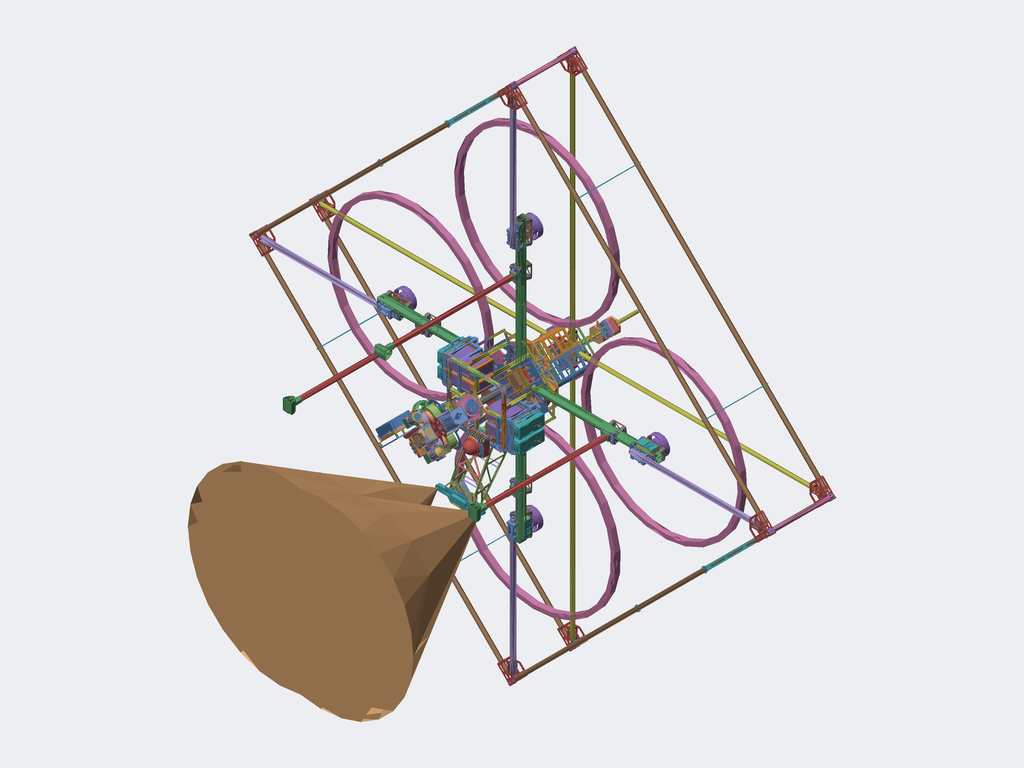Assembly | SolidWorks | 199 different items | 580 placed
Parts list (item | name | quantity | parent item | size | volume | features):
1 | 3D_PCB2_2025-12-14.step (subassembly) | x1 | - | - | - | -
2 | (subassembly) | x2 | in 9 | 27.581 x 78.075 x 26.95 mm | 6505 mm3 | -
3 | (subassembly) | x1 | in 16 | 62 x 54.7 x 76 mm | 57730 mm3 | -
4 | (subassembly) | x1 | in 14 | 113.2 x 36 x 73.2 mm | 73752 mm3 | -
5 | (subassembly) | x1 | in 16 | 72.737 x 60.097 x 64.874 mm | 142272 mm3 | -
6 | (subassembly) | x1 | in 16 | 60.743 x 60.049 x 12 mm | 6986 mm3 | -
7 | (subassembly) | x1 | in 16 | 852.82 x 786 x 692.82 mm | 107026744 mm3 | -
8 | (subassembly) | x1 | in 14 | - | - | -
9 | (subassembly) | x2 | in 16 | - | 914521 mm3 | features InContextFeatHolder 1
10 | (subassembly) | x1 | - | - | - | features InContextFeatHolder 2
11 | (subassembly) | x1 | - | - | - | features CompositeCurve 1
12 | (subassembly) | x1 | in 10 | 110.5 x 147.904 x 41 mm | 42458 mm3 | -
13 | (subassembly) | x1 | in 14 | - | 15304 mm3 | -
14 | (subassembly) | x1 | in 10 | - | - | features CenterOfMass 1
15 | (subassembly) | x1 | in 11 | - | 484779 mm3 | -
16 | (subassembly) | x1 | in 11 | - | - | features InContextFeatHolder 6, CompositeCurve 2
17 | (subassembly) | x1 | in 16 | 113.626 x 72.5 x 130.8 mm | 166546 mm3 | -
18 | BM02B-GHS-TBT.stp | x1 | - | - | - | -
19 | BM04B-GHS-TBT.stp | x1 | - | - | - | -
20 | Board~NjeS_1.step | x1 | - | - | - | -
21 | BottomSilkscreen~NjeS_1.step | x1 | - | - | - | -
22 | - | x1 | in 10 | 16 x 46 x 46 mm | 10417 mm3 | features ICE 6, CirPattern 2, Cut 1, Fillet 1, RefAxis 1, Revolution 1
23 | - | x1 | in 6 | 60 x 60 x 3 mm | 6153 mm3 | features Extrusion 1
24 | - | x32 | in 16 | 36 x 18 x 10 mm | 2888 mm3 | features Fillet 4, Extrusion 1, ICE 1
25 | - | x4 | in 16 | 36 x 3 x 88 mm | 5789 mm3 | features Fillet 3, Extrusion 1, ICE 1
26 | - | x1 | in 16 | 54 x 9.4 x 47.569 mm | 2533 mm3 | features ICE 6, Fillet 2, BossThin 1, Chamfer 1, CirPattern 1, Extrusion 1, MirrorPattern 1, Rib 1
27 | - | x1 | in 16 | 153.518 x 1.5 x 153.518 mm | 7437 mm3 | features Fillet 4, Extrusion 1, ICE 1
28 | - | x2 | in 16 | 194.5 x 58 x 2 mm | 4743 mm3 | features Fillet 5, ICE 2, Chamfer 1, Extrusion 1
29 | - | x2 | in 16 | 24 x 58 x 6.5 mm | 2190 mm3 | features ICE 2, Extrusion 1, Fillet 1
30 | - | x4 | in 16 | 24 x 31 x 24 mm | 4448 mm3 | features Extrusion 1, ICE 1
31 | - | x4 | in 16 | 137.074 x 6.5 x 56.497 mm | 3888 mm3 | features Fillet 5, ICE 3, Extrusion 1
32 | - | x4 | in 2 | 25 x 20.4 x 5.4 mm | 1256 mm3 | features ICE 2, Chamfer 1, Extrusion 1, Fillet 1
33 | - | x1 | in 10 | 22 x 68 x 68 mm | 23228 mm3 | features ICE 6, Fillet 2, BossThin 1, Chamfer 1, CirPattern 1, Cut 1, RefAxis 1, Revolution 1
34 | - | x1 | in 16 | - | 27564 mm3 | features BaseBody 46, ICE 1
35 | - | x1 | in 16 | 76 x 15.652 x 219.462 mm | 48611 mm3 | features BaseBody 13, Revolution 2, ICE 1
36 | - | x1 | in 16 | 45.5 x 41.918 x 59.598 mm | 18797 mm3 | features BaseBody 3, 3DProfileFeature 2, ICE 1, MoveCopyBody 1, NetBlend 1, RefAxis 1, Revolution 1, Sweep 1
37 | - | x1 | in 16 | 66.65 x 61 x 41.1 mm | 16016 mm3 | features ICE 15, Fillet 6, Chamfer 2, Extrusion 1, MirrorPattern 1, RevCut 1, Revolution 1
38 | - | x1 | in 16 | 20 x 140 x 20 mm | 8357 mm3 | features Extrusion 1
39 | - | x4 | in 6 | 6.928 x 6 x 12 mm | 208.267 mm3 | features ICE 2, Extrusion 1
40 | - | x1 | in 16 | 182.976 x 151.8 x 144 mm | 82758 mm3 | features Fillet 17, ICE 10, Extrusion 1, MirrorPattern 1
41 | - | x1 | in 16 | 255.002 x 2 x 157 mm | 8812 mm3 | features Extrusion 1
42 | - | x1 | in 16 | 120.4 x 151.9 x 56.149 mm | 26782 mm3 | features ICE 3, Fillet 2, Emboss 1, Extrusion 1
43 | - | x3 | in 16 | 23.98 x 1 x 7 mm | 119.201 mm3 | features Extrusion 1
44 | - | x1 | in 10 | 76.5 x 63 x 2 mm | 4222 mm3 | features Fillet 4, ICE 4, Extrusion 1
45 | - | x1 | in 16 | 238 x 19 x 238 mm | 66674 mm3 | features ICE 9, Fillet 5, MirrorPattern 3, Extrusion 1
46 | - | x4 | in 16 | 44 x 19 x 68 mm | 11985 mm3 | features ICE 11, Fillet 7, MirrorPattern 3, Extrusion 1
47 | - | x4 | in 16 | 6.889 x 27.8 x 58 mm | 3675 mm3 | features ICE 2, Extrusion 1, Fillet 1
48 | - | x4 | in 9 | 44.3 x 134.791 x 101.5 mm | 420051 mm3 | features BaseBody 9, CenterOfMass 1
49 | - | x96 | in 15, 16 | 17 x 8 x 7 mm | 450.526 mm3 | features Extrusion 1, ICE 1
50 | - | x4 | in 15 | 14 x 14 x 926.63 mm | 19619 mm3 | features Extrusion 1, ICE 1
51 | - | x4 | in 16 | 12 x 12 x 508 mm | 22307 mm3 | features ICE 2, Extrusion 1
52 | - | x4 | in 15 | 12 x 4.8 x 42 mm | 1272 mm3 | features Extrusion 1, Fillet 1
53 | - | x4 | in 16 | 36 x 2 x 88 mm | 3130 mm3 | features Fillet 3, Extrusion 1, ICE 1
54 | - | x4 | in 16 | 40.135 x 16 x 48 mm | 9698 mm3 | features Fillet 4, ICE 4, MirrorPattern 2, Chamfer 1, Extrusion 1
55 | - | x1 | in 10 | 1.5 x 15.6 x 46.4 mm | 731.985 mm3 | features ICE 2, Extrusion 1, Fillet 1
56 | - | x4 | in 16 | 26.5 x 4 x 46.5 mm | 1746 mm3 | features Fillet 3, Extrusion 1
57 | - | x8 | in 15 | 14 x 14 x 1336 mm | 28300 mm3 | features Extrusion 1, ICE 1
58 | - | x4 | in 15 | 12 x 246.5 x 12 mm | 4438 mm3 | features Extrusion 1, ICE 1
59 | - | x8 | in 15 | 26.2 x 17 x 16.2 mm | 2329 mm3 | features Extrusion 1, Fillet 1, ICE 1
60 | - | x2 | in 7 | 2 x 173.5 x 218.5 mm | 10390 mm3 | features ICE 2, Extrusion 1, Fillet 1
61 | - | x6 | in 16 | 31 x 1.5 x 31 mm | 483.32 mm3 | features Fillet 2, Extrusion 1
62 | - | x1 | in 11 | 54.12 x 67 x 69.4 mm | 103995 mm3 | features ICE 6, CirPattern 1, Extrusion 1, HoleWzd 1, MirrorPattern 1, RefAxis 1, Revolution 1
63 | - | x2 | in 9 | 66.8 x 2 x 116.5 mm | 8063 mm3 | features Fillet 3, Chamfer 2, ICE 2, Extrusion 1, HoleWzd 1
64 | - | x1 | in 16 | 85.6 x 68.6 x 1.5 mm | 2523 mm3 | features Fillet 4, Extrusion 1
65 | - | x12 | in 16 | 5 x 5 x 5.95 mm | 71.919 mm3 | features Extrusion 1
66 | - | x1 | in 10 | 3 x 126.828 x 52 mm | 8428 mm3 | features ICE 3, Fillet 2, Extrusion 1
67 | - | x4 | in 16 | 8 x 8 x 55 mm | 1480 mm3 | features Extrusion 1, ICE 1
68 | - | x5 | in 16 | 18 x 1.5 x 24 mm | 359.817 mm3 | features Extrusion 1, Fillet 1
69 | - | x1 | in 16 | 88.56 x 3 x 88.56 mm | 9081 mm3 | features Fillet 3, Extrusion 1, ICE 1
70 | - | x4 | in 16 | 8 x 8 x 185 mm | 4954 mm3 | features ICE 4, Extrusion 1
71 | - | x6 | in 16 | 8 x 152 x 8 mm | 4129 mm3 | features ICE 5, Extrusion 1
72 | - | x12 | in 16 | 24 x 26 x 1.5 mm | 427.683 mm3 | features Fillet 2, Extrusion 1
73 | - | x4 | in 16 | 16 x 475 x 16 mm | 22384 mm3 | features ExtruThin 1
74 | - | x4 | in 16 | 35 x 1.5 x 51 mm | 1129 mm3 | features Fillet 4, Extrusion 1
75 | - | x4 | in 16 | 36 x 3 x 52 mm | 2909 mm3 | features Fillet 3, Extrusion 1, ICE 1
76 | - | x4 | in 9 | 8 x 16.45 x 3 mm | 362.772 mm3 | features Extrusion 1, Fillet 1
77 | - | x1 | in 10 | 68.8 x 54.5 x 2 mm | 2944 mm3 | features Fillet 6, ICE 5, Extrusion 1
78 | - | x4 | in 16 | 6.2 x 8 x 6.2 mm | 177.186 mm3 | features Extrusion 1
79 | - | x1 | in 10 | 3 x 126.828 x 59 mm | 11105 mm3 | features Fillet 3, ICE 2, Extrusion 1, HoleWzd 1
80 | - | x1 | in 10 | 41 x 5 x 41 mm | 2352 mm3 | features BossThin 2, Extrusion 1
81 | - | x1 | in 10 | 72 x 57.8 x 2 mm | 3745 mm3 | features Fillet 3, Extrusion 1
82 | - | x1 | in 14 | - | 22684 mm3 | features BaseBody 8
83 | - | x21 | in 7, 16 | 10 x 10 x 6 mm | 263.588 mm3 | features ICE 2, Extrusion 1
84 | - | x1 | in 14 | 43.4 x 42.4 x 109.827 mm | 92437 mm3 | features BaseBody 32, Revolution 2
85 | - | x1 | in 8 | - | - | features RefSurface 185, BaseBody 6, Revolution 1
86 | - | x1 | in 4 | 113.2 x 26 x 73.2 mm | 44105 mm3 | features BaseBody 1
87 | - | x1 | in 4 | 113.2 x 10 x 73.2 mm | 29648 mm3 | features BaseBody 1
88 | - | x1 | in 10 | 3 x 39.6 x 39.6 mm | 1466 mm3 | features RefAxis 2, CirPattern 1, Extrusion 1, Fillet 1, RevCut 1
89 | - | x1 | in 14 | 30.418 x 30.418 x 18 mm | 3548 mm3 | features ICE 6, Chamfer 2, CoordSys 1, Extrusion 1, Fillet 1, HoleWzd 1
90 | - | x1 | in 10 | 116.779 x 6.9 x 81.5 mm | 10389 mm3 | features Fillet 6, ICE 4, Extrusion 1, MirrorPattern 1, PLine 1, Shell 1
91 | - | x1 | in 16 | 120 x 1.5 x 120 mm | 5507 mm3 | features Fillet 3, Extrusion 1, ICE 1
92 | - | x1 | in 10 | 33 x 6 x 33 mm | 2032 mm3 | features Fillet 2, Extrusion 1, HoleWzd 1, ICE 1, Shell 1
93 | - | x2 | in 10 | 11.407 x 34.229 x 3 mm | 770.437 mm3 | features Extrusion 1
94 | - | x4 | in 16 | 610 x 20 x 610 mm | 578980 mm3 | features Extrusion 1
95 | - | x2 | in 14 | 10 x 10 x 6 mm | 454.401 mm3 | features ICE 3, Extrusion 1
96 | - | x2 | in 10 | 32.2 x 53 x 53 mm | 55104 mm3 | features ICE 1, MBimport 1
97 | - | x4 | in 10 | 7 x 4.6 x 5.312 mm | 93.915 mm3 | features Extrusion 1, HoleWzd 1
98 | - | x1 | in 14 | 3 x 82 x 209.4 mm | 18688 mm3 | features ICE 4, Fillet 3, Extrusion 1
99 | - | x1 | in 14 | 3 x 41.5 x 70.75 mm | 4779 mm3 | features Fillet 3, HoleWzd 2, ICE 2, Extrusion 1
100 | - | x1 | in 14 | 115.25 x 2 x 250.4 mm | 18165 mm3 | features Fillet 3, ICE 2, Chamfer 1, Extrusion 1
101 | - | x1 | in 14 | 153.25 x 2 x 236.9 mm | 13689 mm3 | features Fillet 4, ICE 3, Chamfer 1, Extrusion 1
102 | - | x1 | in 16 | 32 x 31 x 32 mm | 3496 mm3 | features ICE 3, Extrusion 1, Fillet 1
103 | - | x8 | in 15 | 20.2 x 237.5 x 2 mm | 4160 mm3 | features Extrusion 1, Fillet 1
104 | - | x1 | in 14 | 1.5 x 82 x 122 mm | 5369 mm3 | features ICE 2, Extrusion 1, Fillet 1
105 | - | x1 | in 12 | 110.5 x 119.181 x 41 mm | 34590 mm3 | features Fillet 19, ICE 17, Revolution 5, RevCut 2, Extrusion 1
106 | - | x6 | in 10 | 5 x 7 x 7 mm | 152.21 mm3 | features Extrusion 1
107 | - | x1 | in 14 | 43.074 x 29.627 x 49.814 mm | 7359 mm3 | features ICE 15, Fillet 6, Chamfer 5, MirrorPattern 3, RevCut 1, Revolution 1
108 | - | x1 | in 10 | 28 x 38.187 x 37 mm | 8059 mm3 | features ICE 13, Fillet 7, MirrorPattern 4, Extrusion 1
109 | - | x1 | in 14 | 22 x 6.4 x 36 mm | 2076 mm3 | features Fillet 2, Extrusion 1
110 | - | x1 | in 10 | 7 x 35 x 35 mm | 4074 mm3 | features Extrusion 1
111 | - | x2 | in 14 | 21 x 60 x 60 mm | 34134 mm3 | features BaseBody 2
112 | - | x1 | in 10 | 2 x 39.8 x 56 mm | 2062 mm3 | features Fillet 4, Extrusion 1, ICE 1, MirrorPattern 1
113 | - | x1 | in 8 | 151 x 16.5 x 48 mm | 33794 mm3 | features ICE 7, Fillet 6, Extrusion 1, HoleWzd 1
114 | - | x1 | in 14 | 45 x 41.44 x 106.5 mm | 25458 mm3 | features ICE 25, Chamfer 5, HoleWzd 5, Fillet 2, Attribute 1, CenterOfMass 1, Extrusion 1
115 | - | x4 | in 14 | 12 x 5 x 5 mm | 150.796 mm3 | features Extrusion 1
116 | - | x1 | in 14 | 60 x 57.271 x 3 mm | 4694 mm3 | features Fillet 3, RefAxis 2, RevCut 2, Extrusion 1, ICE 1
117 | - | x2 | in 14 | 5 x 40 x 5 mm | 502.655 mm3 | features Extrusion 1
118 | - | x1 | in 10 | 63 x 3 x 66 mm | 7046 mm3 | features Fillet 5, ICE 2, Extrusion 1, HoleWzd 1
119 | - | x1 | in 16 | - | - | features BaseBody 479
120 | - | x1 | in 17 | 81.787 x 85.8 x 7 mm | 16789 mm3 | features ICE 4, Extrusion 1
121 | - | x4 | in 17 | 5 x 18 x 5 mm | 226.195 mm3 | features Extrusion 1
122 | - | x1 | in 17 | 113.626 x 130.8 x 26.5 mm | 67573 mm3 | features ICE 42, Fillet 29, Chamfer 4, Extrusion 1, RevCut 1, SweepCut 1
123 | - | x1 | in 17 | 49.123 x 20 x 51.245 mm | 9173 mm3 | features Chamfer 2, ICE 2, Blend 1, BlendCut 1, Fillet 1
124 | - | x1 | in 17 | 106.727 x 2 x 65 mm | 6307 mm3 | features Fillet 3, Extrusion 1
125 | - | x1 | in 17 | 34 x 11 x 34 mm | 4612 mm3 | features ICE 2, Chamfer 1, Extrusion 1, HoleWzd 1
126 | - | x1 | in 7 | 93.2 x 1.5 x 88.2 mm | 3552 mm3 | features Fillet 2, Extrusion 1
127 | - | x1 | in 10 | 57 x 46 x 57 mm | 102676 mm3 | features BaseBody 10
128 | - | x3 | in 7 | 93.2 x 1.5 x 14 mm | 783.785 mm3 | features Fillet 2, Extrusion 1
129 | - | x1 | in 7 | 135.6 x 2 x 90.853 mm | 6413 mm3 | features Fillet 3, Extrusion 1, ICE 1
130 | - | x1 | in 8 | 42 x 8.717 x 42 mm | 6163 mm3 | features ICE 3, Extrusion 1, Fillet 1
131 | - | x2 | in 10 | 11.6 x 11.6 x 4 mm | 257.334 mm3 | features Extrusion 1, ICE 1
132 | - | x2 | in 16 | 6.466 x 7 x 5.6 mm | 137.276 mm3 | features Extrusion 1
133 | - | x1 | in 16 | 41.82 x 2 x 41.82 mm | 2968 mm3 | features Extrusion 1, Fillet 1
134 | - | x1 | in 16 | 12 x 400 x 12 mm | 25005 mm3 | features ICE 2, Extrusion 1
135 | - | x2 | in 7 | 72 x 8 x 1 mm | 471.693 mm3 | features Extrusion 1
136 | - | x1 | in 7 | 852.82 x 692.82 x 610 mm | 106933293 mm3 | features Revolution 2, Cut 1, Extrusion 1, Fillet 1, HoleWzd 1, ICE 1
137 | - | x1 | in 7 | 78.5 x 53.5 x 14 mm | 58364 mm3 | features Extrusion 1, Fillet 1
138 | - | x2 | in 14 | 42 x 44.967 x 43.4 mm | 38568 mm3 | features BaseBody 24, RefSurface 18
139 | - | x4 | in 16 | 21 x 6 x 6 mm | 586.354 mm3 | features Extrusion 1, ICE 1
140 | - | x4 | in 16 | 5 x 150 x 5 mm | 1885 mm3 | features Extrusion 1
141 | - | x3 | in 16 | 5 x 14 x 5 mm | 175.929 mm3 | features Extrusion 1
142 | - | x14 | in 16 | 5 x 40 x 5 mm | 502.655 mm3 | features Extrusion 1
143 | - | x4 | in 3 | 5 x 40 x 5 mm | 502.655 mm3 | features Extrusion 1
144 | - | x3 | in 10 | 6.8 x 6 x 6.8 mm | 169.646 mm3 | features Extrusion 1
145 | - | x4 | in 16 | 5 x 12 x 5 mm | 150.796 mm3 | features Extrusion 1
146 | - | x4 | in 16 | 61 x 30.44 x 15.6 mm | 7234 mm3 | features BaseBody 6
147 | - | x1 | in 17 | 36 x 53 x 53.058 mm | 61188 mm3 | features BaseBody 19
148 | - | x1 | in 16 | 68.5 x 2 x 43 mm | 2475 mm3 | features Extrusion 1, Fillet 1, HoleWzd 1
149 | - | x10 | in 10 | 22 x 8 x 8 mm | 1182 mm3 | features Extrusion 1, ICE 1
150 | - | x2 | in 8 | - | - | features BaseBody 4, RefSurface 1
151 | - | x1 | in 8 | 33 x 42.54 x 33 mm | 18425 mm3 | features BaseBody 16
152 | - | x1 | in 8 | 33 x 39.959 x 33.465 mm | 16722 mm3 | features BaseBody 33
153 | - | x1 | in 3 | 48.33 x 11.1 x 28.16 mm | 12571 mm3 | features ICE 7, Fillet 2, Chamfer 1, Extrusion 1
154 | - | x1 | in 3 | 58.21 x 16.91 x 38.92 mm | 32464 mm3 | features ICE 92, Chamfer 2, CenterOfMass 1, Extrusion 1, Fillet 1
155 | - | x1 | in 3 | 61.2 x 4.4 x 75.2 mm | 6161 mm3 | features Fillet 3, ICE 2, Extrusion 1
156 | - | x1 | in 3 | 62 x 2 x 76 mm | 4523 mm3 | features Extrusion 1, Fillet 1
157 | - | x1 | in 12 | 39.5 x 28.723 x 28 mm | 7867 mm3 | features ICE 9, Fillet 4, MirrorPattern 4, Extrusion 1, Revolution 1
158 | - | x1 | in 10 | 9 x 9 x 21.5 mm | 469.445 mm3 | features ICE 2, Extrusion 1, StudWizard 1
159 | - | x1 | in 16 | 45 x 2 x 15 mm | 1215 mm3 | features Extrusion 1, Fillet 1, HoleWzd 1
160 | - | x10 | in 14 | 21 x 6 x 6 mm | 586.354 mm3 | features Extrusion 1, ICE 1
161 | - | x1 | in 16 | 42.5 x 4 x 29.485 mm | 1175 mm3 | features Extrusion 1, Fillet 1, HoleWzd 1
162 | - | x1 | in 16 | 8.158 x 9.6 x 23.257 mm | 1128 mm3 | features Chamfer 2, Extrusion 1, ICE 1
163 | - | x4 | in 16 | 72 x 72 x 33.4 mm | 24620 mm3 | features MBimport 1
164 | - | x4 | in 16 | 33 x 48.321 x 40 mm | 10302 mm3 | features ICE 2, Extrusion 1
165 | - | x16 | in 15 | 70.368 x 2 x 70.368 mm | 4319 mm3 | features Fillet 4, Extrusion 1
166 | - | x1 | in 16 | 121 x 2 x 43.639 mm | 2162 mm3 | features Extrusion 1, Fillet 1
167 | - | x1 | in 16 | 262.722 x 2 x 262.722 mm | 50644 mm3 | features Fillet 6, ICE 2, Extrusion 1
168 | - | x1 | in 16 | 262.722 x 2 x 262.722 mm | 67464 mm3 | features Fillet 7, Extrusion 1, ICE 1
169 | - | x2 | in 9 | 119.7 x 110.236 x 66.6 mm | 59225 mm3 | features ICE 28, Chamfer 5, Fillet 5, MirrorPattern 2, Extrusion 1
170 | - | x4 | in 16 | 20 x 30 x 475 mm | 40009 mm3 | features ICE 3, Fillet 2, Extrusion 1
171 | - | x1 | in 8 | 42 x 6.5 x 42 mm | 5775 mm3 | features ICE 2, Extrusion 1, Fillet 1
172 | CENTER_DISTRIBUTION_BOARD.stp | x1 | - | - | - | -
173 | MID-360_4_1.stp | x1 | - | - | - | -
174 | MID-360_4_2.stp | x1 | - | - | - | -
175 | MID-360_4_3.stp | x1 | - | - | - | -
176 | MID-360_4_4.stp | x1 | - | - | - | -
177 | MID-360_4_5.stp | x1 | - | - | - | -
178 | MID-360_4_6.stp | x1 | - | - | - | -
179 | MID-360_4_7.stp | x1 | - | - | - | -
180 | MID-360_4_ASM.stp (subassembly) | x1 | - | - | - | -
181 | - | x1 | - | - | - | -
182 | SHELL_DOWN.stp | x1 | - | - | - | -
183 | SHELL_UP.stp | x1 | - | - | - | -
184 | SM02B-GHS-TB.stp | x1 | - | - | - | -
185 | TH_2P-XT60PW-F~TH_2P-XT60PW-F~NjeS_1.step | x1 | - | - | - | -
186 | TopSilkscreen~NjeS_1.step | x1 | - | - | - | -
187 | U1~TH_2P-XT60PW-F~TH_2P-XT60PW-F~NjeS_1.step (subassembly) | x1 | - | - | - | -
188 | XT30UPB-F_3D_DRAWING_ASM.stp (subassembly) | x1 | - | - | - | -
189 | XT30UPB-F_ASM.stp (subassembly) | x1 | - | - | - | -
190 | XT30UPB-F_SJ.stp | x1 | - | - | - | -
191 | - | x1 | - | - | - | -
192 | - | x1 | - | - | - | -
193 | - | x1 | - | - | - | -
194 | - | x1 | - | - | - | -
195 | - | x1 | - | - | - | -
196 | (subassembly) | x1 | - | - | - | -
197 | eBom-FreeParts.stp | x1 | - | - | - | -
198 | mid-360-asm.stp (subassembly) | x1 | - | - | - | -
199 |  ESC Adapter Plate.stp (subassembly) | x1 | - | - | - | -
Mates (type | each side: item.copy, entity, surface, feature), first 410 of 1199 lines:
In the top assembly
Coincident | 69.1 face plane Boss-Extrude 1 | 80.1 face plane Boss-Extrude 1
Concentric | 69.1 face cylinder Boss-Extrude 1 | 90.1 face cylinder Boss-Extrude 1 | 2 times
In subassembly 11
Concentric | 51.1 face cylinder Cut-Extrude 1 | 52.1 face cylinder Boss-Extrude 1
Concentric | 51.1 face cylinder Cut-Extrude 1 | 165.1 face cylinder Boss-Extrude 1
Coincident | 51.2 face plane Boss-Extrude 1 | 165.2 face plane Boss-Extrude 1
Concentric | 134.1 face cylinder Boss-Extrude 1 | 62.1 face cylinder Boss-Extrude 1
DistanceDim | 62.1 face plane Boss-Extrude 1 | 27.1 face plane Boss-Extrude 1
Parallel | 27.1 face plane Boss-Extrude 1 | 62.1 face plane Boss-Extrude 1
In subassembly 15
Concentric | 165.3 face cylinder Boss-Extrude 1 | 59.1 face cylinder Boss-Extrude 1
Coincident | 165.3 face plane Boss-Extrude 1 | 59.1 face plane Boss-Extrude 1
Concentric | 59.1 face cylinder Boss-Extrude 1 | 165.4 face cylinder Boss-Extrude 1 | 2 times
Coincident | 59.1 face plane Boss-Extrude 1 | 165.4 face plane Boss-Extrude 1
Coincident | 165.4 face plane Boss-Extrude 1 | 49.1 face plane Boss-Extrude 1
Concentric | 165.4 face cylinder Boss-Extrude 1 | 49.1 face cylinder Cut-Extrude 1
Parallel | 165.4 face plane Boss-Extrude 1 | 49.1 face plane Boss-Extrude 1
Coincident | 165.3 face plane Boss-Extrude 1 | 49.2 face plane Boss-Extrude 1
Concentric | 165.3 face cylinder Boss-Extrude 1 | 49.2 face cylinder Cut-Extrude 1
Coincident | 49.1 face plane Boss-Extrude 1 | 49.2 face plane Boss-Extrude 1
Concentric | 165.4 face cylinder Boss-Extrude 1 | 57.1 face cylinder Cut-Extrude 1 | 2 times
Concentric | 49.2 face cylinder Boss-Extrude 1 | 57.1 face cylinder Boss-Extrude 2
Concentric | 165.4 face cylinder Boss-Extrude 1 | 49.3 face cylinder Cut-Extrude 1
Concentric | 49.3 face cylinder Boss-Extrude 1 | 57.1 face cylinder Boss-Extrude 2
Concentric | 165.3 face cylinder Boss-Extrude 1 | 49.4 face cylinder Cut-Extrude 1
Concentric | 49.4 face cylinder Boss-Extrude 1 | 57.1 face cylinder Boss-Extrude 2
Concentric | 165.3 face cylinder Boss-Extrude 1 | 49.5 face cylinder Cut-Extrude 1
Coincident | 165.3 face plane Boss-Extrude 1 | 49.5 face plane Boss-Extrude 1
Parallel | 165.3 face plane Boss-Extrude 1 | 49.5 face plane Boss-Extrude 1
Concentric | 165.4 face cylinder Boss-Extrude 1 | 49.6 face cylinder Cut-Extrude 1
Coincident | 165.4 face plane Boss-Extrude 1 | 49.6 face plane Boss-Extrude 1
Coincident | 49.6 face plane Boss-Extrude 1 | 49.5 face plane Boss-Extrude 1
Concentric | 165.4 face cylinder Boss-Extrude 1 | 57.2 face cylinder Cut-Extrude 1
Concentric | 49.5 face cylinder Boss-Extrude 1 | 57.2 face cylinder Boss-Extrude 2
Concentric | 165.3 face cylinder Boss-Extrude 1 | 49.7 face cylinder Cut-Extrude 1
Concentric | 49.7 face cylinder Boss-Extrude 1 | 57.2 face cylinder Boss-Extrude 2
Concentric | 165.4 face cylinder Boss-Extrude 1 | 49.8 face cylinder Cut-Extrude 1
Concentric | 49.8 face cylinder Boss-Extrude 1 | 57.2 face cylinder Boss-Extrude 2
Concentric | 165.4 face cylinder Boss-Extrude 1 | 49.9 face cylinder Cut-Extrude 1
Coincident | 165.4 face plane Boss-Extrude 1 | 49.9 face plane Boss-Extrude 1
Parallel | 165.4 face plane Boss-Extrude 1 | 49.9 face plane Boss-Extrude 1
Coincident | 165.3 face plane Boss-Extrude 1 | 49.10 face plane Boss-Extrude 1
Concentric | 165.3 face cylinder Boss-Extrude 1 | 49.10 face cylinder Cut-Extrude 1
Coincident | 49.9 face plane Boss-Extrude 1 | 49.10 face plane Boss-Extrude 1
Coincident | 165.5 face plane Boss-Extrude 1 | 59.2 face plane Boss-Extrude 1
Concentric | 165.5 face cylinder Boss-Extrude 1 | 59.2 face cylinder Boss-Extrude 1
Coincident | 165.6 face plane Boss-Extrude 1 | 59.2 face plane Boss-Extrude 1
Concentric | 165.6 face cylinder Boss-Extrude 1 | 59.2 face cylinder Boss-Extrude 1 | 2 times
Concentric | 165.6 face cylinder Boss-Extrude 1 | 49.11 face cylinder Cut-Extrude 1
Coincident | 165.6 face plane Boss-Extrude 1 | 49.11 face plane Boss-Extrude 1
Parallel | 165.6 face plane Boss-Extrude 1 | 49.11 face plane Boss-Extrude 1
Concentric | 57.1 face cylinder Cut-Extrude 1 | 165.6 face cylinder Boss-Extrude 1
Concentric | 57.1 face cylinder Boss-Extrude 2 | 49.11 face cylinder Boss-Extrude 1
Concentric | 165.5 face cylinder Boss-Extrude 1 | 49.12 face cylinder Cut-Extrude 1
Concentric | 57.1 face cylinder Boss-Extrude 2 | 49.12 face cylinder Boss-Extrude 1
Concentric | 165.6 face cylinder Boss-Extrude 1 | 49.13 face cylinder Cut-Extrude 1
Concentric | 57.1 face cylinder Boss-Extrude 2 | 49.13 face cylinder Boss-Extrude 1
Concentric | 165.5 face cylinder Boss-Extrude 1 | 49.14 face cylinder Cut-Extrude 1
Concentric | 57.1 face cylinder Boss-Extrude 2 | 49.14 face cylinder Boss-Extrude 1
Concentric | 165.6 face cylinder Boss-Extrude 1 | 49.15 face cylinder Cut-Extrude 1
Coincident | 165.6 face plane Boss-Extrude 1 | 49.15 face plane Boss-Extrude 1
Parallel | 165.6 face plane Boss-Extrude 1 | 49.15 face plane Boss-Extrude 1
Concentric | 165.5 face cylinder Boss-Extrude 1 | 49.16 face cylinder Cut-Extrude 1
Coincident | 165.5 face plane Boss-Extrude 1 | 49.16 face plane Boss-Extrude 1
Coincident | 49.15 face plane Boss-Extrude 1 | 49.16 face plane Boss-Extrude 1
Concentric | 49.15 face cylinder Boss-Extrude 1 | 57.3 face cylinder Boss-Extrude 2
Concentric | 165.6 face cylinder Boss-Extrude 1 | 49.17 face cylinder Cut-Extrude 1
Concentric | 57.3 face cylinder Boss-Extrude 2 | 49.17 face cylinder Boss-Extrude 1
Concentric | 165.5 face cylinder Boss-Extrude 1 | 49.18 face cylinder Cut-Extrude 1
Concentric | 57.3 face cylinder Boss-Extrude 2 | 49.18 face cylinder Boss-Extrude 1
Concentric | 165.6 face cylinder Boss-Extrude 1 | 57.3 face cylinder Cut-Extrude 1
Concentric | 165.6 face cylinder Boss-Extrude 1 | 49.19 face cylinder Cut-Extrude 1
Coincident | 165.6 face plane Boss-Extrude 1 | 49.19 face plane Boss-Extrude 1
Parallel | 165.6 face plane Boss-Extrude 1 | 49.19 face plane Boss-Extrude 1
Concentric | 165.5 face cylinder Boss-Extrude 1 | 49.20 face cylinder Cut-Extrude 1
Concentric | 49.19 face cylinder Boss-Extrude 1 | 49.20 face cylinder Boss-Extrude 1
Concentric | 165.5 face cylinder Boss-Extrude 1 | 49.21 face cylinder Cut-Extrude 1
Coincident | 165.5 face plane Boss-Extrude 1 | 49.21 face plane Boss-Extrude 1 | 2 times
Concentric | 165.6 face cylinder Boss-Extrude 1 | 49.22 face cylinder Cut-Extrude 1
Concentric | 49.21 face cylinder Boss-Extrude 1 | 49.22 face cylinder Boss-Extrude 1
Concentric | 165.4 face cylinder Boss-Extrude 1 | 49.23 face cylinder Cut-Extrude 1
Coincident | 165.4 face plane Boss-Extrude 1 | 49.23 face plane Boss-Extrude 1 | 2 times
Concentric | 165.3 face cylinder Boss-Extrude 1 | 49.24 face cylinder Cut-Extrude 1
Concentric | 49.23 face cylinder Boss-Extrude 1 | 49.24 face cylinder Boss-Extrude 1
Concentric | 165.7 face cylinder Boss-Extrude 1 | 59.3 face cylinder Boss-Extrude 1
Coincident | 165.7 face plane Boss-Extrude 1 | 59.3 face plane Boss-Extrude 1
Concentric | 165.8 face cylinder Boss-Extrude 1 | 59.3 face cylinder Boss-Extrude 1 | 2 times
Coincident | 165.8 face plane Boss-Extrude 1 | 59.3 face plane Boss-Extrude 1
Coincident | 165.8 face plane Boss-Extrude 1 | 49.25 face plane Boss-Extrude 1
Concentric | 165.8 face cylinder Boss-Extrude 1 | 49.25 face cylinder Cut-Extrude 1
Parallel | 165.8 face plane Boss-Extrude 1 | 49.25 face plane Boss-Extrude 1
Coincident | 165.7 face plane Boss-Extrude 1 | 49.26 face plane Boss-Extrude 1
Concentric | 165.7 face cylinder Boss-Extrude 1 | 49.26 face cylinder Cut-Extrude 1
Coincident | 49.26 face plane Boss-Extrude 1 | 49.25 face plane Boss-Extrude 1
Concentric | 165.8 face cylinder Boss-Extrude 1 | 49.27 face cylinder Cut-Extrude 1
Concentric | 165.7 face cylinder Boss-Extrude 1 | 49.28 face cylinder Cut-Extrude 1
Concentric | 165.7 face cylinder Boss-Extrude 1 | 49.29 face cylinder Cut-Extrude 1
Coincident | 165.7 face plane Boss-Extrude 1 | 49.29 face plane Boss-Extrude 1
Parallel | 165.7 face plane Boss-Extrude 1 | 49.29 face plane Boss-Extrude 1
Concentric | 165.8 face cylinder Boss-Extrude 1 | 49.30 face cylinder Cut-Extrude 1
Coincident | 165.8 face plane Boss-Extrude 1 | 49.30 face plane Boss-Extrude 1
Coincident | 49.29 face plane Boss-Extrude 1 | 49.30 face plane Boss-Extrude 1
Concentric | 165.7 face cylinder Boss-Extrude 1 | 49.31 face cylinder Cut-Extrude 1
Concentric | 165.8 face cylinder Boss-Extrude 1 | 49.32 face cylinder Cut-Extrude 1
Concentric | 165.8 face cylinder Boss-Extrude 1 | 49.33 face cylinder Cut-Extrude 1
Coincident | 165.8 face plane Boss-Extrude 1 | 49.33 face plane Boss-Extrude 1
Parallel | 165.8 face plane Boss-Extrude 1 | 49.33 face plane Boss-Extrude 1
Coincident | 165.7 face plane Boss-Extrude 1 | 49.34 face plane Boss-Extrude 1
Concentric | 165.7 face cylinder Boss-Extrude 1 | 49.34 face cylinder Cut-Extrude 1
Coincident | 49.34 face plane Boss-Extrude 1 | 49.33 face plane Boss-Extrude 1
Concentric | 165.8 face cylinder Boss-Extrude 1 | 49.35 face cylinder Cut-Extrude 1
Coincident | 165.8 face plane Boss-Extrude 1 | 49.35 face plane Boss-Extrude 1 | 2 times
Concentric | 165.7 face cylinder Boss-Extrude 1 | 49.36 face cylinder Cut-Extrude 1
Concentric | 49.36 face cylinder Boss-Extrude 1 | 49.35 face cylinder Boss-Extrude 1
Concentric | 57.2 face cylinder Cut-Extrude 1 | 165.8 face cylinder Boss-Extrude 1 | 2 times
Coincident | 165.7 face plane Boss-Extrude 1 | 49.28 face plane Boss-Extrude 1
Concentric | 57.2 face cylinder Boss-Extrude 2 | 49.25 face cylinder Boss-Extrude 1
Concentric | 57.2 face cylinder Boss-Extrude 2 | 49.27 face cylinder Boss-Extrude 1
Concentric | 57.2 face cylinder Boss-Extrude 2 | 49.28 face cylinder Boss-Extrude 1
Coincident | 165.7 face plane Boss-Extrude 1 | 49.31 face plane Boss-Extrude 1
Concentric | 49.29 face cylinder Boss-Extrude 1 | 49.31 face cylinder Boss-Extrude 1
Concentric | 49.31 face cylinder Boss-Extrude 1 | 49.32 face cylinder Boss-Extrude 1
Concentric | 49.32 face cylinder Cut-Extrude 1 | 57.4 face cylinder Cut-Extrude 1
Concentric | 49.32 face cylinder Boss-Extrude 1 | 57.4 face cylinder Boss-Extrude 2
Concentric | 165.9 face cylinder Boss-Extrude 1 | 59.4 face cylinder Boss-Extrude 1
Coincident | 165.9 face plane Boss-Extrude 1 | 59.4 face plane Boss-Extrude 1
Concentric | 165.10 face cylinder Boss-Extrude 1 | 59.4 face cylinder Boss-Extrude 1 | 2 times
Coincident | 165.10 face plane Boss-Extrude 1 | 59.4 face plane Boss-Extrude 1
Coincident | 165.10 face plane Boss-Extrude 1 | 49.37 face plane Boss-Extrude 1
Concentric | 165.10 face cylinder Boss-Extrude 1 | 49.37 face cylinder Cut-Extrude 1
Parallel | 165.10 face plane Boss-Extrude 1 | 49.37 face plane Boss-Extrude 1
Coincident | 165.9 face plane Boss-Extrude 1 | 49.38 face plane Boss-Extrude 1
Concentric | 165.9 face cylinder Boss-Extrude 1 | 49.38 face cylinder Cut-Extrude 1
Coincident | 49.37 face plane Boss-Extrude 1 | 49.38 face plane Boss-Extrude 1
Concentric | 165.10 face cylinder Boss-Extrude 1 | 49.39 face cylinder Cut-Extrude 1
Concentric | 165.9 face cylinder Boss-Extrude 1 | 49.40 face cylinder Cut-Extrude 1
Concentric | 165.9 face cylinder Boss-Extrude 1 | 49.41 face cylinder Cut-Extrude 1
Coincident | 165.9 face plane Boss-Extrude 1 | 49.41 face plane Boss-Extrude 1
Parallel | 165.9 face plane Boss-Extrude 1 | 49.41 face plane Boss-Extrude 1
Concentric | 165.10 face cylinder Boss-Extrude 1 | 49.42 face cylinder Cut-Extrude 1
Coincident | 165.10 face plane Boss-Extrude 1 | 49.42 face plane Boss-Extrude 1
Coincident | 49.41 face plane Boss-Extrude 1 | 49.42 face plane Boss-Extrude 1
Concentric | 165.9 face cylinder Boss-Extrude 1 | 49.43 face cylinder Cut-Extrude 1
Concentric | 165.10 face cylinder Boss-Extrude 1 | 49.44 face cylinder Cut-Extrude 1
Concentric | 165.10 face cylinder Boss-Extrude 1 | 49.45 face cylinder Cut-Extrude 1
Coincident | 165.10 face plane Boss-Extrude 1 | 49.45 face plane Boss-Extrude 1
Parallel | 165.10 face plane Boss-Extrude 1 | 49.45 face plane Boss-Extrude 1
Coincident | 165.9 face plane Boss-Extrude 1 | 49.46 face plane Boss-Extrude 1
Concentric | 165.9 face cylinder Boss-Extrude 1 | 49.46 face cylinder Cut-Extrude 1
Coincident | 49.45 face plane Boss-Extrude 1 | 49.46 face plane Boss-Extrude 1
Concentric | 165.10 face cylinder Boss-Extrude 1 | 49.47 face cylinder Cut-Extrude 1
Coincident | 165.10 face plane Boss-Extrude 1 | 49.47 face plane Boss-Extrude 1 | 2 times
Concentric | 165.9 face cylinder Boss-Extrude 1 | 49.48 face cylinder Cut-Extrude 1
Concentric | 49.48 face cylinder Boss-Extrude 1 | 49.47 face cylinder Boss-Extrude 1
Coincident | 165.9 face plane Boss-Extrude 1 | 49.40 face plane Boss-Extrude 1
Coincident | 165.9 face plane Boss-Extrude 1 | 49.43 face plane Boss-Extrude 1
Concentric | 49.43 face cylinder Boss-Extrude 1 | 49.41 face cylinder Boss-Extrude 1
Concentric | 49.44 face cylinder Boss-Extrude 1 | 49.43 face cylinder Boss-Extrude 1
Concentric | 57.4 face cylinder Cut-Extrude 1 | 165.10 face cylinder Boss-Extrude 1 | 2 times
Concentric | 57.4 face cylinder Boss-Extrude 2 | 49.37 face cylinder Boss-Extrude 1
Concentric | 57.4 face cylinder Boss-Extrude 2 | 49.39 face cylinder Boss-Extrude 1
Concentric | 57.4 face cylinder Boss-Extrude 2 | 49.40 face cylinder Boss-Extrude 1
Concentric | 57.3 face cylinder Cut-Extrude 1 | 49.44 face cylinder Cut-Extrude 1
Concentric | 57.3 face cylinder Boss-Extrude 2 | 49.44 face cylinder Boss-Extrude 1
Concentric | 59.4 face cylinder Boss-Extrude 1 | 58.1 face cylinder Boss-Extrude 1
Concentric | 59.5 face cylinder Boss-Extrude 1 | 165.11 face cylinder Boss-Extrude 1
Concentric | 59.5 face cylinder Boss-Extrude 1 | 165.12 face cylinder Boss-Extrude 1
Coincident | 59.5 face plane Boss-Extrude 1 | 165.11 face plane Boss-Extrude 1
Coincident | 59.5 face plane Boss-Extrude 1 | 165.12 face plane Boss-Extrude 1
Concentric | 58.1 face cylinder Boss-Extrude 1 | 165.11 face cylinder Boss-Extrude 1
Concentric | 49.49 face cylinder Cut-Extrude 1 | 165.11 face cylinder Boss-Extrude 1
Coincident | 49.37 face plane Boss-Extrude 1 | 49.49 face plane Boss-Extrude 1
Coincident | 49.49 face plane Boss-Extrude 1 | 165.11 face plane Boss-Extrude 1
Concentric | 49.50 face cylinder Cut-Extrude 1 | 165.12 face cylinder Boss-Extrude 1
Concentric | 49.49 face cylinder Boss-Extrude 1 | 49.50 face cylinder Boss-Extrude 1
Concentric | 49.51 face cylinder Boss-Extrude 1 | 49.52 face cylinder Boss-Extrude 1
Concentric | 165.11 face cylinder Boss-Extrude 1 | 49.52 face cylinder Cut-Extrude 1
Coincident | 49.39 face plane Boss-Extrude 1 | 49.52 face plane Boss-Extrude 1
Coincident | 165.11 face plane Boss-Extrude 1 | 49.52 face plane Boss-Extrude 1
Concentric | 165.12 face cylinder Boss-Extrude 1 | 49.51 face cylinder Cut-Extrude 1
Concentric | 49.53 face cylinder Boss-Extrude 1 | 49.54 face cylinder Boss-Extrude 1
Concentric | 165.11 face cylinder Boss-Extrude 1 | 49.54 face cylinder Cut-Extrude 1
Coincident | 49.44 face plane Boss-Extrude 1 | 49.54 face plane Boss-Extrude 1
Coincident | 165.11 face plane Boss-Extrude 1 | 49.54 face plane Boss-Extrude 1
Concentric | 165.12 face cylinder Boss-Extrude 1 | 49.53 face cylinder Cut-Extrude 1
Concentric | 49.55 face cylinder Boss-Extrude 1 | 49.56 face cylinder Boss-Extrude 1
Concentric | 165.11 face cylinder Boss-Extrude 1 | 49.56 face cylinder Cut-Extrude 1
Coincident | 49.41 face plane Boss-Extrude 1 | 49.56 face plane Boss-Extrude 1
Coincident | 165.11 face plane Boss-Extrude 1 | 49.56 face plane Boss-Extrude 1
Concentric | 165.12 face cylinder Boss-Extrude 1 | 49.55 face cylinder Cut-Extrude 1
Concentric | 59.4 face cylinder Cut-Extrude 1 | 58.1 face cylinder Cut-Extrude 1
Concentric | 165.11 face cylinder Boss-Extrude 1 | 52.2 face cylinder Boss-Extrude 1
Coincident | 165.11 face plane Boss-Extrude 1 | 52.2 face plane Boss-Extrude 1 | 2 times
Concentric | 59.6 face cylinder Boss-Extrude 1 | 165.13 face cylinder Boss-Extrude 1
Concentric | 165.14 face cylinder Boss-Extrude 1 | 59.6 face cylinder Boss-Extrude 1
Coincident | 59.6 face plane Boss-Extrude 1 | 165.13 face plane Boss-Extrude 1
Coincident | 165.14 face plane Boss-Extrude 1 | 59.6 face plane Boss-Extrude 1
Concentric | 165.13 face cylinder Boss-Extrude 1 | 58.2 face cylinder Boss-Extrude 1
Concentric | 49.57 face cylinder Cut-Extrude 1 | 165.13 face cylinder Boss-Extrude 1
Coincident | 49.57 face plane Boss-Extrude 1 | 165.13 face plane Boss-Extrude 1
Concentric | 165.14 face cylinder Boss-Extrude 1 | 49.58 face cylinder Cut-Extrude 1
Concentric | 49.57 face cylinder Boss-Extrude 1 | 49.58 face cylinder Boss-Extrude 1
Concentric | 49.59 face cylinder Boss-Extrude 1 | 49.60 face cylinder Boss-Extrude 1
Concentric | 49.59 face cylinder Cut-Extrude 1 | 165.13 face cylinder Boss-Extrude 1
Coincident | 49.59 face plane Boss-Extrude 1 | 165.13 face plane Boss-Extrude 1
Concentric | 165.14 face cylinder Boss-Extrude 1 | 49.60 face cylinder Cut-Extrude 1
Concentric | 49.61 face cylinder Boss-Extrude 1 | 49.62 face cylinder Boss-Extrude 1
Concentric | 165.13 face cylinder Boss-Extrude 1 | 49.62 face cylinder Cut-Extrude 1
Coincident | 165.13 face plane Boss-Extrude 1 | 49.62 face plane Boss-Extrude 1
Concentric | 165.14 face cylinder Boss-Extrude 1 | 49.61 face cylinder Cut-Extrude 1
Concentric | 49.63 face cylinder Boss-Extrude 1 | 49.64 face cylinder Boss-Extrude 1
Concentric | 165.13 face cylinder Boss-Extrude 1 | 49.63 face cylinder Cut-Extrude 1
Coincident | 165.13 face plane Boss-Extrude 1 | 49.63 face plane Boss-Extrude 1
Concentric | 165.14 face cylinder Boss-Extrude 1 | 49.64 face cylinder Cut-Extrude 1
Concentric | 165.13 face cylinder Boss-Extrude 1 | 52.3 face cylinder Boss-Extrude 1
Coincident | 165.13 face plane Boss-Extrude 1 | 52.3 face plane Boss-Extrude 1 | 2 times
Concentric | 59.2 face cylinder Boss-Extrude 1 | 58.2 face cylinder Boss-Extrude 1
Coincident | 49.16 face plane Boss-Extrude 1 | 49.57 face plane Boss-Extrude 1
Coincident | 49.17 face plane Boss-Extrude 1 | 49.59 face plane Boss-Extrude 1
Coincident | 49.12 face plane Boss-Extrude 1 | 49.62 face plane Boss-Extrude 1
Coincident | 49.14 face plane Boss-Extrude 1 | 49.63 face plane Boss-Extrude 1
Concentric | 59.2 face cylinder Cut-Extrude 1 | 58.2 face cylinder Cut-Extrude 1
Concentric | 59.7 face cylinder Boss-Extrude 1 | 165.15 face cylinder Boss-Extrude 1
Coincident | 59.7 face plane Boss-Extrude 1 | 165.15 face plane Boss-Extrude 1
Concentric | 165.15 face cylinder Boss-Extrude 1 | 58.3 face cylinder Boss-Extrude 1
Concentric | 49.65 face cylinder Cut-Extrude 1 | 165.15 face cylinder Boss-Extrude 1
Coincident | 49.65 face plane Boss-Extrude 1 | 165.15 face plane Boss-Extrude 1
Concentric | 49.66 face cylinder Cut-Extrude 1 | 165.15 face cylinder Boss-Extrude 1
Coincident | 49.66 face plane Boss-Extrude 1 | 165.15 face plane Boss-Extrude 1
Concentric | 165.15 face cylinder Boss-Extrude 1 | 49.67 face cylinder Cut-Extrude 1
Coincident | 165.15 face plane Boss-Extrude 1 | 49.67 face plane Boss-Extrude 1
Concentric | 165.15 face cylinder Boss-Extrude 1 | 49.68 face cylinder Cut-Extrude 1
Coincident | 165.15 face plane Boss-Extrude 1 | 49.68 face plane Boss-Extrude 1
Concentric | 165.15 face cylinder Boss-Extrude 1 | 52.4 face cylinder Boss-Extrude 1
Coincident | 165.15 face plane Boss-Extrude 1 | 52.4 face plane Boss-Extrude 1 | 2 times
Concentric | 59.1 face cylinder Boss-Extrude 1 | 58.3 face cylinder Boss-Extrude 1
Coincident | 49.3 face plane Boss-Extrude 1 | 49.65 face plane Boss-Extrude 1
Coincident | 49.1 face plane Boss-Extrude 1 | 49.66 face plane Boss-Extrude 1
Coincident | 49.7 face plane Boss-Extrude 1 | 49.67 face plane Boss-Extrude 1
Coincident | 49.5 face plane Boss-Extrude 1 | 49.68 face plane Boss-Extrude 1
Concentric | 59.1 face cylinder Cut-Extrude 1 | 58.3 face cylinder Cut-Extrude 1
Concentric | 165.8 face cylinder Boss-Extrude 1 | 58.4 face cylinder Boss-Extrude 1
Concentric | 59.3 face cylinder Cut-Extrude 1 | 58.4 face cylinder Cut-Extrude 1
Concentric | 58.4 face cylinder Boss-Extrude 1 | 165.16 face cylinder Boss-Extrude 1
Coincident | 59.8 face plane Boss-Extrude 1 | 165.16 face plane Boss-Extrude 1
Concentric | 165.16 face cylinder Boss-Extrude 1 | 49.69 face cylinder Cut-Extrude 1
Concentric | 57.5 face cylinder Boss-Extrude 2 | 49.69 face cylinder Boss-Extrude 1
Concentric | 165.16 face cylinder Boss-Extrude 1 | 49.70 face cylinder Cut-Extrude 1
Concentric | 57.5 face cylinder Boss-Extrude 2 | 49.70 face cylinder Boss-Extrude 1
Concentric | 165.16 face cylinder Boss-Extrude 1 | 49.71 face cylinder Cut-Extrude 1
Concentric | 165.16 face cylinder Boss-Extrude 1 | 49.72 face cylinder Cut-Extrude 1
Concentric | 58.3 face cylinder Boss-Extrude 1 | 165.17 face cylinder Boss-Extrude 1
Coincident | 59.7 face plane Boss-Extrude 1 | 165.17 face plane Boss-Extrude 1
Concentric | 165.17 face cylinder Boss-Extrude 1 | 49.73 face cylinder Cut-Extrude 1
Concentric | 49.65 face cylinder Boss-Extrude 1 | 49.73 face cylinder Boss-Extrude 1
Concentric | 165.17 face cylinder Boss-Extrude 1 | 49.74 face cylinder Cut-Extrude 1
Concentric | 49.66 face cylinder Boss-Extrude 1 | 49.74 face cylinder Boss-Extrude 1
Concentric | 165.17 face cylinder Boss-Extrude 1 | 49.75 face cylinder Cut-Extrude 1
Concentric | 49.67 face cylinder Boss-Extrude 1 | 49.75 face cylinder Boss-Extrude 1
Concentric | 165.17 face cylinder Boss-Extrude 1 | 49.76 face cylinder Cut-Extrude 1
Concentric | 49.68 face cylinder Boss-Extrude 1 | 49.76 face cylinder Boss-Extrude 1
Concentric | 57.5 face cylinder Cut-Extrude 1 | 165.16 face cylinder Boss-Extrude 1
Concentric | 165.17 face cylinder Boss-Extrude 1 | 57.6 face cylinder Cut-Extrude 1
Concentric | 49.65 face cylinder Boss-Extrude 1 | 57.6 face cylinder Boss-Extrude 2
Concentric | 165.14 face cylinder Boss-Extrude 1 | 57.7 face cylinder Cut-Extrude 1
Concentric | 49.57 face cylinder Boss-Extrude 1 | 57.7 face cylinder Boss-Extrude 2
Concentric | 165.12 face cylinder Boss-Extrude 1 | 57.8 face cylinder Cut-Extrude 1
Concentric | 49.49 face cylinder Boss-Extrude 1 | 57.8 face cylinder Boss-Extrude 2
Concentric | 49.24 face cylinder Boss-Extrude 1 | 50.1 face cylinder Boss-Extrude 1
Concentric | 165.4 face cylinder Boss-Extrude 1 | 50.1 face cylinder Cut-Extrude 1
Concentric | 49.21 face cylinder Boss-Extrude 1 | 50.2 face cylinder Boss-Extrude 1
Concentric | 165.6 face cylinder Boss-Extrude 1 | 50.2 face cylinder Cut-Extrude 1
Concentric | 49.48 face cylinder Boss-Extrude 1 | 50.3 face cylinder Boss-Extrude 1
Concentric | 165.10 face cylinder Boss-Extrude 1 | 50.3 face cylinder Cut-Extrude 1
Concentric | 49.36 face cylinder Boss-Extrude 1 | 50.4 face cylinder Boss-Extrude 1
Concentric | 165.8 face cylinder Boss-Extrude 1 | 50.4 face cylinder Cut-Extrude 1
Concentric | 59.7 face cylinder Cut-Extrude 1 | 58.3 face cylinder Cut-Extrude 1
Concentric | 59.8 face cylinder Cut-Extrude 1 | 58.4 face cylinder Cut-Extrude 1
Concentric | 58.1 face cylinder Cut-Extrude 1 | 59.5 face cylinder Cut-Extrude 1
Concentric | 59.6 face cylinder Cut-Extrude 1 | 58.2 face cylinder Cut-Extrude 1
Concentric | 57.1 face cylinder Boss-Extrude 2 | 103.1 face cylinder Boss-Extrude 1
Parallel | 165.14 face plane Boss-Extrude 1 | 103.1 face plane Boss-Extrude 1
DistanceDim | 165.6 face plane Boss-Extrude 1 | 103.1 face plane Boss-Extrude 1
Concentric | 103.1 face cylinder Boss-Extrude 1 | 103.2 face cylinder Boss-Extrude 1
Coincident | 103.1 face plane Boss-Extrude 1 | 103.2 face plane Boss-Extrude 1
DistanceDim | 103.2 face plane Boss-Extrude 1 | 165.15 face plane Boss-Extrude 1
Concentric | 165.11 face cylinder Boss-Extrude 1 | 49.51 face cylinder Cut-Extrude 1
Concentric | 57.2 face cylinder Boss-Extrude 2 | 103.3 face cylinder Boss-Extrude 1
Parallel | 165.17 face plane Boss-Extrude 1 | 103.3 face plane Boss-Extrude 1
DistanceDim | 165.15 face plane Boss-Extrude 1 | 103.3 face plane Boss-Extrude 1
Concentric | 165.18 face cylinder Boss-Extrude 1 | 49.77 face cylinder Cut-Extrude 1
Coincident | 165.18 face plane Boss-Extrude 1 | 49.77 face plane Boss-Extrude 1
Concentric | 165.18 face cylinder Boss-Extrude 1 | 49.78 face cylinder Cut-Extrude 1
Coincident | 165.18 face plane Boss-Extrude 1 | 49.78 face plane Boss-Extrude 1
Concentric | 165.18 face cylinder Boss-Extrude 1 | 49.79 face cylinder Cut-Extrude 1
Coincident | 165.18 face plane Boss-Extrude 1 | 49.79 face plane Boss-Extrude 1
Concentric | 165.18 face cylinder Boss-Extrude 1 | 49.80 face cylinder Cut-Extrude 1
Coincident | 165.18 face plane Boss-Extrude 1 | 49.80 face plane Boss-Extrude 1
Concentric | 165.18 face cylinder Boss-Extrude 1 | 52.5 face cylinder Boss-Extrude 1
Coincident | 165.18 face plane Boss-Extrude 1 | 52.5 face plane Boss-Extrude 1 | 2 times
Concentric | 58.4 face cylinder Boss-Extrude 1 | 165.18 face cylinder Boss-Extrude 1
Concentric | 57.5 face cylinder Boss-Extrude 2 | 49.78 face cylinder Boss-Extrude 1
Concentric | 57.5 face cylinder Boss-Extrude 2 | 49.76 face cylinder Boss-Extrude 1
Concentric | 57.5 face cylinder Boss-Extrude 2 | 103.4 face cylinder Boss-Extrude 1
Coincident | 103.3 face plane Boss-Extrude 1 | 103.4 face plane Boss-Extrude 1
DistanceDim | 103.4 face plane Boss-Extrude 1 | 165.18 face plane Boss-Extrude 1
Concentric | 57.8 face cylinder Boss-Extrude 2 | 49.80 face cylinder Boss-Extrude 1
Concentric | 57.8 face cylinder Boss-Extrude 2 | 49.79 face cylinder Boss-Extrude 1
Concentric | 57.5 face cylinder Boss-Extrude 2 | 49.77 face cylinder Boss-Extrude 1
Concentric | 49.71 face cylinder Boss-Extrude 1 | 57.8 face cylinder Boss-Extrude 2
Concentric | 49.72 face cylinder Boss-Extrude 1 | 57.8 face cylinder Boss-Extrude 2
Concentric | 57.8 face cylinder Boss-Extrude 2 | 103.5 face cylinder Boss-Extrude 1
DistanceDim | 103.5 face plane Boss-Extrude 1 | 165.18 face plane Boss-Extrude 1
Parallel | 165.18 face plane Boss-Extrude 1 | 103.5 face plane Boss-Extrude 1
Concentric | 57.8 face cylinder Boss-Extrude 2 | 103.6 face cylinder Boss-Extrude 1
Coincident | 103.5 face plane Boss-Extrude 1 | 103.6 face plane Boss-Extrude 1
DistanceDim | 103.6 face plane Boss-Extrude 1 | 165.11 face plane Boss-Extrude 1
Concentric | 57.7 face cylinder Boss-Extrude 2 | 103.7 face cylinder Boss-Extrude 1
Parallel | 165.11 face plane Boss-Extrude 1 | 103.7 face plane Boss-Extrude 1
DistanceDim | 103.7 face plane Boss-Extrude 1 | 165.11 face plane Boss-Extrude 1
Concentric | 57.7 face cylinder Boss-Extrude 2 | 103.8 face cylinder Boss-Extrude 1
Coincident | 103.7 face plane Boss-Extrude 1 | 103.8 face plane Boss-Extrude 1
DistanceDim | 165.13 face plane Boss-Extrude 1 | 103.8 face plane Boss-Extrude 1
In subassembly 16
Concentric | 45.1 face cylinder Boss-Extrude 3 | 170.1 face cylinder Cut-Extrude 1 | 2 times
Coincident | 45.1 face plane Cut-Extrude 2 | 170.1 face plane Boss-Extrude 1
Coincident | 45.1 face plane Cut-Extrude 2 | 170.2 face plane Boss-Extrude 1
Concentric | 45.1 face cylinder Boss-Extrude 3 | 46.1 face cylinder Boss-Extrude 3
Concentric | 170.1 face cylinder Cut-Extrude 1 | 46.1 face cylinder Boss-Extrude 3
Coincident | 170.1 face plane Boss-Extrude 1 | 46.1 face plane Cut-Extrude 2
Concentric | 45.1 face cylinder Boss-Extrude 3 | 170.3 face cylinder Cut-Extrude 1 | 2 times
Coincident | 45.1 face plane Mirror 2 | 170.3 face plane Boss-Extrude 1
Concentric | 45.1 face cylinder Boss-Extrude 3 | 170.4 face cylinder Cut-Extrude 1 | 2 times
Coincident | 45.1 face plane Mirror 2 | 170.4 face plane Boss-Extrude 1
Concentric | 45.1 face cylinder Boss-Extrude 3 | 46.2 face cylinder Boss-Extrude 3 | 2 times
Coincident | 170.4 face plane Boss-Extrude 1 | 46.2 face plane Cut-Extrude 2
Concentric | 170.2 face cylinder Cut-Extrude 1 | 46.3 face cylinder Boss-Extrude 3 | 2 times
Coincident | 170.2 face plane Boss-Extrude 1 | 46.3 face plane Cut-Extrude 2
Concentric | 170.3 face cylinder Cut-Extrude 1 | 46.4 face cylinder Boss-Extrude 3 | 2 times
Coincident | 170.3 face plane Boss-Extrude 1 | 46.4 face plane Cut-Extrude 2
Concentric | 46.4 face cylinder Boss-Extrude 3 | 168.1 face cylinder Boss-Extrude 1
Concentric | 46.1 face cylinder Boss-Extrude 3 | 168.1 face cylinder Boss-Extrude 1
Concentric | 163.1 face cylinder mad-m6c12-eee.stp<1> | 25.1 face cylinder Boss-Extrude 1 | 2 times
Coincident | 163.1 face plane mad-m6c12-eee.stp<1> | 25.1 face plane Boss-Extrude 1
Coincident | 163.1 face plane mad-m6c12-eee.stp<1> | 94.1 face plane Boss-Extrude 1
Concentric | 163.1 face cylinder mad-m6c12-eee.stp<1> | 94.1 face cylinder Boss-Extrude 1
Concentric | 25.1 face cylinder Boss-Extrude 1 | 24.1 face cylinder Boss-Extrude 1 | 2 times
Coincident | 25.1 face plane Boss-Extrude 1 | 24.1 face plane Boss-Extrude 1
Concentric | 25.1 face cylinder Boss-Extrude 1 | 24.2 face cylinder Boss-Extrude 1 | 2 times
Coincident | 25.1 face plane Boss-Extrude 1 | 24.2 face plane Boss-Extrude 1
Concentric | 170.2 face cylinder Cut-Extrude 1 | 24.2 face cylinder Boss-Extrude 1
Concentric | 170.2 face cylinder Cut-Extrude 1 | 24.1 face cylinder Boss-Extrude 1
Coincident | 170.2 face plane Boss-Extrude 1 | 24.1 face plane Cut-Extrude 1
Concentric | 163.2 face cylinder mad-m6c12-eee.stp<1> | 25.2 face cylinder Boss-Extrude 1 | 2 times
Coincident | 163.2 face plane mad-m6c12-eee.stp<1> | 25.2 face plane Boss-Extrude 1
Coincident | 163.2 face plane mad-m6c12-eee.stp<1> | 94.2 face plane Boss-Extrude 1
Concentric | 163.2 face cylinder mad-m6c12-eee.stp<1> | 94.2 face cylinder Boss-Extrude 1
Concentric | 24.3 face cylinder Boss-Extrude 1 | 25.2 face cylinder Boss-Extrude 1 | 2 times
Coincident | 24.3 face plane Boss-Extrude 1 | 25.2 face plane Boss-Extrude 1
Concentric | 24.4 face cylinder Boss-Extrude 1 | 25.2 face cylinder Boss-Extrude 1 | 2 times
Coincident | 24.4 face plane Boss-Extrude 1 | 25.2 face plane Boss-Extrude 1
Concentric | 170.4 face cylinder Cut-Extrude 1 | 24.4 face cylinder Boss-Extrude 1
Concentric | 170.4 face cylinder Cut-Extrude 1 | 24.3 face cylinder Boss-Extrude 1
Coincident | 170.4 face plane Boss-Extrude 1 | 24.3 face plane Cut-Extrude 1
Concentric | 163.3 face cylinder mad-m6c12-eee.stp<1> | 25.3 face cylinder Boss-Extrude 1 | 2 times
Coincident | 163.3 face plane mad-m6c12-eee.stp<1> | 25.3 face plane Boss-Extrude 1
Coincident | 163.3 face plane mad-m6c12-eee.stp<1> | 94.3 face plane Boss-Extrude 1
Concentric | 163.3 face cylinder mad-m6c12-eee.stp<1> | 94.3 face cylinder Boss-Extrude 1
Concentric | 24.5 face cylinder Boss-Extrude 1 | 25.3 face cylinder Boss-Extrude 1 | 2 times
Coincident | 24.5 face plane Boss-Extrude 1 | 25.3 face plane Boss-Extrude 1
Concentric | 24.6 face cylinder Boss-Extrude 1 | 25.3 face cylinder Boss-Extrude 1 | 2 times
Coincident | 24.6 face plane Boss-Extrude 1 | 25.3 face plane Boss-Extrude 1
Concentric | 170.1 face cylinder Cut-Extrude 1 | 24.6 face cylinder Boss-Extrude 1
Concentric | 170.1 face cylinder Cut-Extrude 1 | 24.5 face cylinder Boss-Extrude 1
Coincident | 170.1 face plane Boss-Extrude 1 | 24.5 face plane Cut-Extrude 1
Concentric | 163.4 face cylinder mad-m6c12-eee.stp<1> | 25.4 face cylinder Boss-Extrude 1 | 2 times
Coincident | 163.4 face plane mad-m6c12-eee.stp<1> | 25.4 face plane Boss-Extrude 1
Coincident | 163.4 face plane mad-m6c12-eee.stp<1> | 94.4 face plane Boss-Extrude 1
Concentric | 163.4 face cylinder mad-m6c12-eee.stp<1> | 94.4 face cylinder Boss-Extrude 1
Concentric | 24.7 face cylinder Boss-Extrude 1 | 25.4 face cylinder Boss-Extrude 1 | 2 times
Coincident | 24.7 face plane Boss-Extrude 1 | 25.4 face plane Boss-Extrude 1
Concentric | 24.8 face cylinder Boss-Extrude 1 | 25.4 face cylinder Boss-Extrude 1 | 2 times
Coincident | 24.8 face plane Boss-Extrude 1 | 25.4 face plane Boss-Extrude 1
Concentric | 170.3 face cylinder Cut-Extrude 1 | 24.8 face cylinder Boss-Extrude 1
Concentric | 170.3 face cylinder Cut-Extrude 1 | 24.7 face cylinder Boss-Extrude 1
Coincident | 170.3 face plane Boss-Extrude 1 | 24.7 face plane Cut-Extrude 1
Concentric | 170.4 face cylinder Cut-Extrude 2 | 146.1 face cylinder MAD-AMPX-40A  (5-14S).stp-1/12S-40A_ASM_20201102_ASM_ASM_4_ASM_1.stp-1/LY40_ASM_ASM_ASM_ASM_1_ASM_1.stp-1/LY40_ASM_171_ASM_ASM_ASM_1_ASM_1.stp-1/XC108-BOTTOP_78_3_1.stp-1-solid1 | 2 times
Coincident | 170.4 face plane Boss-Extrude 1 | 146.1 face plane MAD-AMPX-40A  (5-14S).stp-1/12S-40A_ASM_20201102_ASM_ASM_4_ASM_1.stp-1/LY40_ASM_ASM_ASM_ASM_1_ASM_1.stp-1/LY40_ASM_171_ASM_ASM_ASM_1_ASM_1.stp-1/XC108-BOTTOP_78_3_1.stp-1-solid1
Coincident | 170.1 face plane Boss-Extrude 1 | 146.2 face plane MAD-AMPX-40A  (5-14S).stp-1/12S-40A_ASM_20201102_ASM_ASM_4_ASM_1.stp-1/LY40_ASM_ASM_ASM_ASM_1_ASM_1.stp-1/LY40_ASM_171_ASM_ASM_ASM_1_ASM_1.stp-1/XC108-BOTTOP_78_3_1.stp-1-solid1
Concentric | 170.1 face cylinder Cut-Extrude 2 | 146.2 face cylinder MAD-AMPX-40A  (5-14S).stp-1/12S-40A_ASM_20201102_ASM_ASM_4_ASM_1.stp-1/LY40_ASM_ASM_ASM_ASM_1_ASM_1.stp-1/LY40_ASM_171_ASM_ASM_ASM_1_ASM_1.stp-1/XC108-BOTTOP_78_3_1.stp-1-solid1 | 2 times
Concentric | 170.2 face cylinder Cut-Extrude 2 | 146.3 face cylinder MAD-AMPX-40A  (5-14S).stp-1/12S-40A_ASM_20201102_ASM_ASM_4_ASM_1.stp-1/LY40_ASM_ASM_ASM_ASM_1_ASM_1.stp-1/LY40_ASM_171_ASM_ASM_ASM_1_ASM_1.stp-1/XC108-BOTTOP_78_3_1.stp-1-solid1 | 2 times
Coincident | 170.2 face plane Boss-Extrude 1 | 146.3 face plane MAD-AMPX-40A  (5-14S).stp-1/12S-40A_ASM_20201102_ASM_ASM_4_ASM_1.stp-1/LY40_ASM_ASM_ASM_ASM_1_ASM_1.stp-1/LY40_ASM_171_ASM_ASM_ASM_1_ASM_1.stp-1/XC108-BOTTOP_78_3_1.stp-1-solid1
Concentric | 170.3 face cylinder Cut-Extrude 2 | 146.4 face cylinder MAD-AMPX-40A  (5-14S).stp-1/12S-40A_ASM_20201102_ASM_ASM_4_ASM_1.stp-1/LY40_ASM_ASM_ASM_ASM_1_ASM_1.stp-1/LY40_ASM_171_ASM_ASM_ASM_1_ASM_1.stp-1/XC108-BOTTOP_78_3_1.stp-1-solid1 | 2 times
Coincident | 170.3 face plane Boss-Extrude 1 | 146.4 face plane MAD-AMPX-40A  (5-14S).stp-1/12S-40A_ASM_20201102_ASM_ASM_4_ASM_1.stp-1/LY40_ASM_ASM_ASM_ASM_1_ASM_1.stp-1/LY40_ASM_171_ASM_ASM_ASM_1_ASM_1.stp-1/XC108-BOTTOP_78_3_1.stp-1-solid1
Concentric | 24.5 face cylinder Boss-Extrude 1 | 24.9 face cylinder Boss-Extrude 1 | 2 times
Coincident | 170.1 face plane Boss-Extrude 1 | 24.9 face plane Cut-Extrude 1
Concentric | 24.6 face cylinder Boss-Extrude 1 | 24.10 face cylinder Boss-Extrude 1 | 2 times
Coincident | 170.1 face plane Boss-Extrude 1 | 24.10 face plane Cut-Extrude 1
Concentric | 24.3 face cylinder Boss-Extrude 1 | 24.11 face cylinder Boss-Extrude 1 | 2 times
Coincident | 170.4 face plane Boss-Extrude 1 | 24.11 face plane Cut-Extrude 1
Concentric | 24.4 face cylinder Boss-Extrude 1 | 24.12 face cylinder Boss-Extrude 1 | 2 times
Coincident | 170.4 face plane Boss-Extrude 1 | 24.12 face plane Cut-Extrude 1
Concentric | 24.9 face cylinder Boss-Extrude 1 | 53.1 face cylinder Boss-Extrude 1
Concentric | 24.10 face cylinder Boss-Extrude 1 | 53.1 face cylinder Boss-Extrude 1
Coincident | 24.10 face plane Boss-Extrude 1 | 53.1 face plane Boss-Extrude 1
Concentric | 56.1 face cylinder Boss-Extrude 1 | 53.1 face cylinder Boss-Extrude 1 | 2 times
Coincident | 56.1 face plane Boss-Extrude 1 | 53.1 face plane Boss-Extrude 1
Concentric | 24.11 face cylinder Boss-Extrude 1 | 53.2 face cylinder Boss-Extrude 1
Concentric | 24.12 face cylinder Boss-Extrude 1 | 53.2 face cylinder Boss-Extrude 1